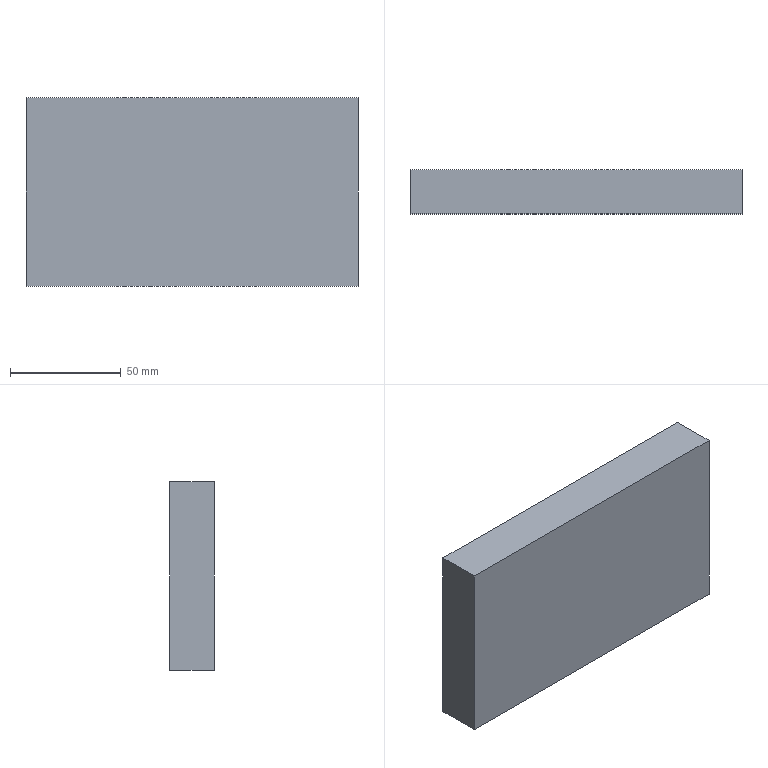Part | NX | features solid 2 | 1 solid | 6 faces | box 150 x 20 x 85 mm | volume 255000 mm3 | plane 6
STEP:
#1=CARTESIAN_POINT('',(-260.,-185.,-70.));
#2=VERTEX_POINT('',#1);
#3=CARTESIAN_POINT('',(-260.,-185.,15.));
#4=VERTEX_POINT('',#3);
#5=CARTESIAN_POINT('',(-260.,-185.,-60.));
#6=DIRECTION('',(0.,0.,1.));
#7=VECTOR('',#6,1000.);
#8=LINE('',#5,#7);
#9=EDGE_CURVE('',#2,#4,#8,.T.);
#10=ORIENTED_EDGE('',*,*,#9,.F.);
#11=CARTESIAN_POINT('',(-260.,-205.,-70.));
#12=VERTEX_POINT('',#11);
#13=CARTESIAN_POINT('',(-260.,-205.,-70.));
#14=DIRECTION('',(0.,1.,0.));
#15=VECTOR('',#14,1000.);
#16=LINE('',#13,#15);
#17=EDGE_CURVE('',#12,#2,#16,.T.);
#18=ORIENTED_EDGE('',*,*,#17,.F.);
#19=CARTESIAN_POINT('',(-260.,-205.,15.));
#20=VERTEX_POINT('',#19);
#21=CARTESIAN_POINT('',(-260.,-205.,-60.));
#22=DIRECTION('',(0.,0.,1.));
#23=VECTOR('',#22,1000.);
#24=LINE('',#21,#23);
#25=EDGE_CURVE('',#12,#20,#24,.T.);
#26=ORIENTED_EDGE('',*,*,#25,.T.);
#27=CARTESIAN_POINT('',(-260.,-205.,15.));
#28=DIRECTION('',(0.,1.,0.));
#29=VECTOR('',#28,1000.);
#30=LINE('',#27,#29);
#31=EDGE_CURVE('',#20,#4,#30,.T.);
#32=ORIENTED_EDGE('',*,*,#31,.T.);
#33=EDGE_LOOP('',(#10,#18,#26,#32));
#34=FACE_BOUND('',#33,.T.);
#35=CARTESIAN_POINT('',(-260.,-205.,-60.));
#36=DIRECTION('',(-1.,0.,0.));
#37=DIRECTION('',(0.,0.,1.));
#38=AXIS2_PLACEMENT_3D('',#35,#36,#37);
#39=PLANE('',#38);
#40=ADVANCED_FACE('',(#34),#39,.T.);
#41=CARTESIAN_POINT('',(-110.,-185.,15.));
#42=VERTEX_POINT('',#41);
#43=CARTESIAN_POINT('',(-95.,-185.,15.));
#44=DIRECTION('',(-1.,0.,0.));
#45=VECTOR('',#44,1000.);
#46=LINE('',#43,#45);
#47=EDGE_CURVE('',#4,#42,#46,.F.);
#48=ORIENTED_EDGE('',*,*,#47,.F.);
#49=ORIENTED_EDGE('',*,*,#31,.F.);
#50=CARTESIAN_POINT('',(-110.,-205.,15.));
#51=VERTEX_POINT('',#50);
#52=CARTESIAN_POINT('',(-95.,-205.,15.));
#53=DIRECTION('',(-1.,0.,0.));
#54=VECTOR('',#53,1000.);
#55=LINE('',#52,#54);
#56=EDGE_CURVE('',#20,#51,#55,.F.);
#57=ORIENTED_EDGE('',*,*,#56,.T.);
#58=CARTESIAN_POINT('',(-110.,-205.,15.));
#59=DIRECTION('',(0.,1.,0.));
#60=VECTOR('',#59,1000.);
#61=LINE('',#58,#60);
#62=EDGE_CURVE('',#51,#42,#61,.T.);
#63=ORIENTED_EDGE('',*,*,#62,.T.);
#64=EDGE_LOOP('',(#48,#49,#57,#63));
#65=FACE_BOUND('',#64,.T.);
#66=CARTESIAN_POINT('',(-95.,-205.,15.));
#67=DIRECTION('',(0.,0.,1.));
#68=DIRECTION('',(1.,0.,0.));
#69=AXIS2_PLACEMENT_3D('',#66,#67,#68);
#70=PLANE('',#69);
#71=ADVANCED_FACE('',(#65),#70,.T.);
#72=CARTESIAN_POINT('',(-110.,-185.,-70.));
#73=VERTEX_POINT('',#72);
#74=CARTESIAN_POINT('',(-110.,-185.,-60.));
#75=DIRECTION('',(0.,0.,1.));
#76=VECTOR('',#75,1000.);
#77=LINE('',#74,#76);
#78=EDGE_CURVE('',#73,#42,#77,.T.);
#79=ORIENTED_EDGE('',*,*,#78,.T.);
#80=ORIENTED_EDGE('',*,*,#62,.F.);
#81=CARTESIAN_POINT('',(-110.,-205.,-70.));
#82=VERTEX_POINT('',#81);
#83=CARTESIAN_POINT('',(-110.,-205.,-60.));
#84=DIRECTION('',(0.,0.,1.));
#85=VECTOR('',#84,1000.);
#86=LINE('',#83,#85);
#87=EDGE_CURVE('',#82,#51,#86,.T.);
#88=ORIENTED_EDGE('',*,*,#87,.F.);
#89=CARTESIAN_POINT('',(-110.,-205.,-70.));
#90=DIRECTION('',(0.,1.,0.));
#91=VECTOR('',#90,1000.);
#92=LINE('',#89,#91);
#93=EDGE_CURVE('',#82,#73,#92,.T.);
#94=ORIENTED_EDGE('',*,*,#93,.T.);
#95=EDGE_LOOP('',(#79,#80,#88,#94));
#96=FACE_BOUND('',#95,.T.);
#97=CARTESIAN_POINT('',(-110.,-205.,-60.));
#98=DIRECTION('',(-1.,0.,0.));
#99=DIRECTION('',(0.,0.,1.));
#100=AXIS2_PLACEMENT_3D('',#97,#98,#99);
#101=PLANE('',#100);
#102=ADVANCED_FACE('',(#96),#101,.F.);
#103=CARTESIAN_POINT('',(-95.,-185.,-70.));
#104=DIRECTION('',(-1.,0.,0.));
#105=VECTOR('',#104,1000.);
#106=LINE('',#103,#105);
#107=EDGE_CURVE('',#73,#2,#106,.T.);
#108=ORIENTED_EDGE('',*,*,#107,.F.);
#109=ORIENTED_EDGE('',*,*,#93,.F.);
#110=CARTESIAN_POINT('',(-95.,-205.,-70.));
#111=DIRECTION('',(-1.,0.,0.));
#112=VECTOR('',#111,1000.);
#113=LINE('',#110,#112);
#114=EDGE_CURVE('',#82,#12,#113,.T.);
#115=ORIENTED_EDGE('',*,*,#114,.T.);
#116=ORIENTED_EDGE('',*,*,#17,.T.);
#117=EDGE_LOOP('',(#108,#109,#115,#116));
#118=FACE_BOUND('',#117,.T.);
#119=CARTESIAN_POINT('',(-95.,-205.,-70.));
#120=DIRECTION('',(0.,0.,-1.));
#121=DIRECTION('',(-1.,0.,0.));
#122=AXIS2_PLACEMENT_3D('',#119,#120,#121);
#123=PLANE('',#122);
#124=ADVANCED_FACE('',(#118),#123,.T.);
#125=ORIENTED_EDGE('',*,*,#25,.F.);
#126=ORIENTED_EDGE('',*,*,#114,.F.);
#127=ORIENTED_EDGE('',*,*,#87,.T.);
#128=ORIENTED_EDGE('',*,*,#56,.F.);
#129=EDGE_LOOP('',(#125,#126,#127,#128));
#130=FACE_BOUND('',#129,.T.);
#131=CARTESIAN_POINT('',(-95.,-205.,-60.));
#132=DIRECTION('',(0.,1.,0.));
#133=DIRECTION('',(0.,0.,1.));
#134=AXIS2_PLACEMENT_3D('',#131,#132,#133);
#135=PLANE('',#134);
#136=ADVANCED_FACE('',(#130),#135,.F.);
#137=ORIENTED_EDGE('',*,*,#9,.T.);
#138=ORIENTED_EDGE('',*,*,#47,.T.);
#139=ORIENTED_EDGE('',*,*,#78,.F.);
#140=ORIENTED_EDGE('',*,*,#107,.T.);
#141=EDGE_LOOP('',(#137,#138,#139,#140));
#142=FACE_BOUND('',#141,.T.);
#143=CARTESIAN_POINT('',(-95.,-185.,-60.));
#144=DIRECTION('',(0.,1.,0.));
#145=DIRECTION('',(0.,0.,1.));
#146=AXIS2_PLACEMENT_3D('',#143,#144,#145);
#147=PLANE('',#146);
#148=ADVANCED_FACE('',(#142),#147,.T.);
#149=CLOSED_SHELL('',(#40,#71,#102,#124,#136,#148));
#150=MANIFOLD_SOLID_BREP('',#149);
#151=(LENGTH_UNIT()NAMED_UNIT(*)SI_UNIT(.MILLI.,.METRE.));
#152=UNCERTAINTY_MEASURE_WITH_UNIT(LENGTH_MEASURE(0.00001),#151,'','');
#153=(NAMED_UNIT(*)PLANE_ANGLE_UNIT()SI_UNIT($,.RADIAN.));
#154=(NAMED_UNIT(*)SI_UNIT($,.STERADIAN.)SOLID_ANGLE_UNIT());
#155=(GEOMETRIC_REPRESENTATION_CONTEXT(3)GLOBAL_UNCERTAINTY_ASSIGNED_CONTEXT((#152))GLOBAL_UNIT_ASSIGNED_CONTEXT((#151,#153,#154))REPRESENTATION_CONTEXT('',''));
#156=ADVANCED_BREP_SHAPE_REPRESENTATION('',(#150),#155);